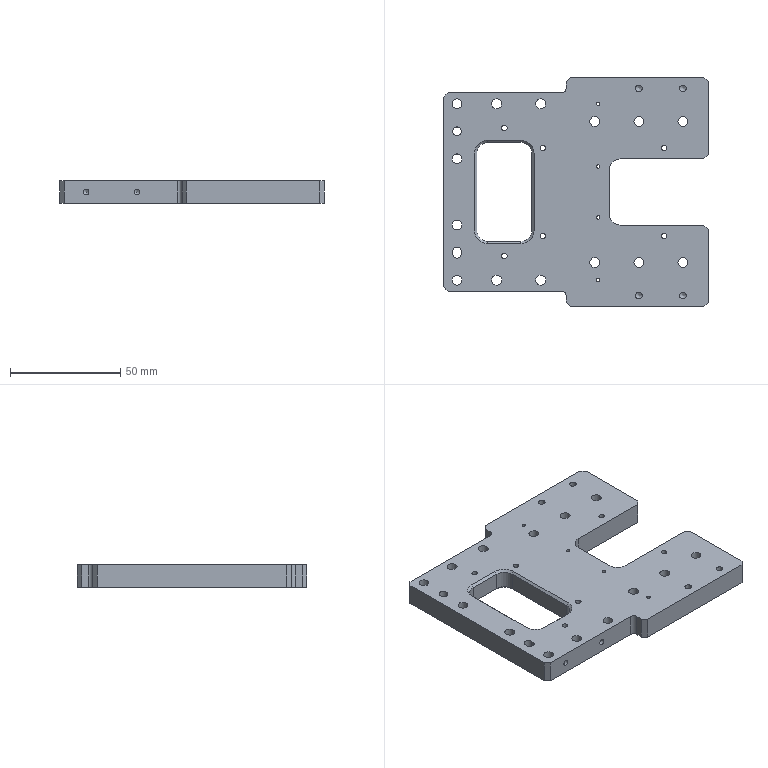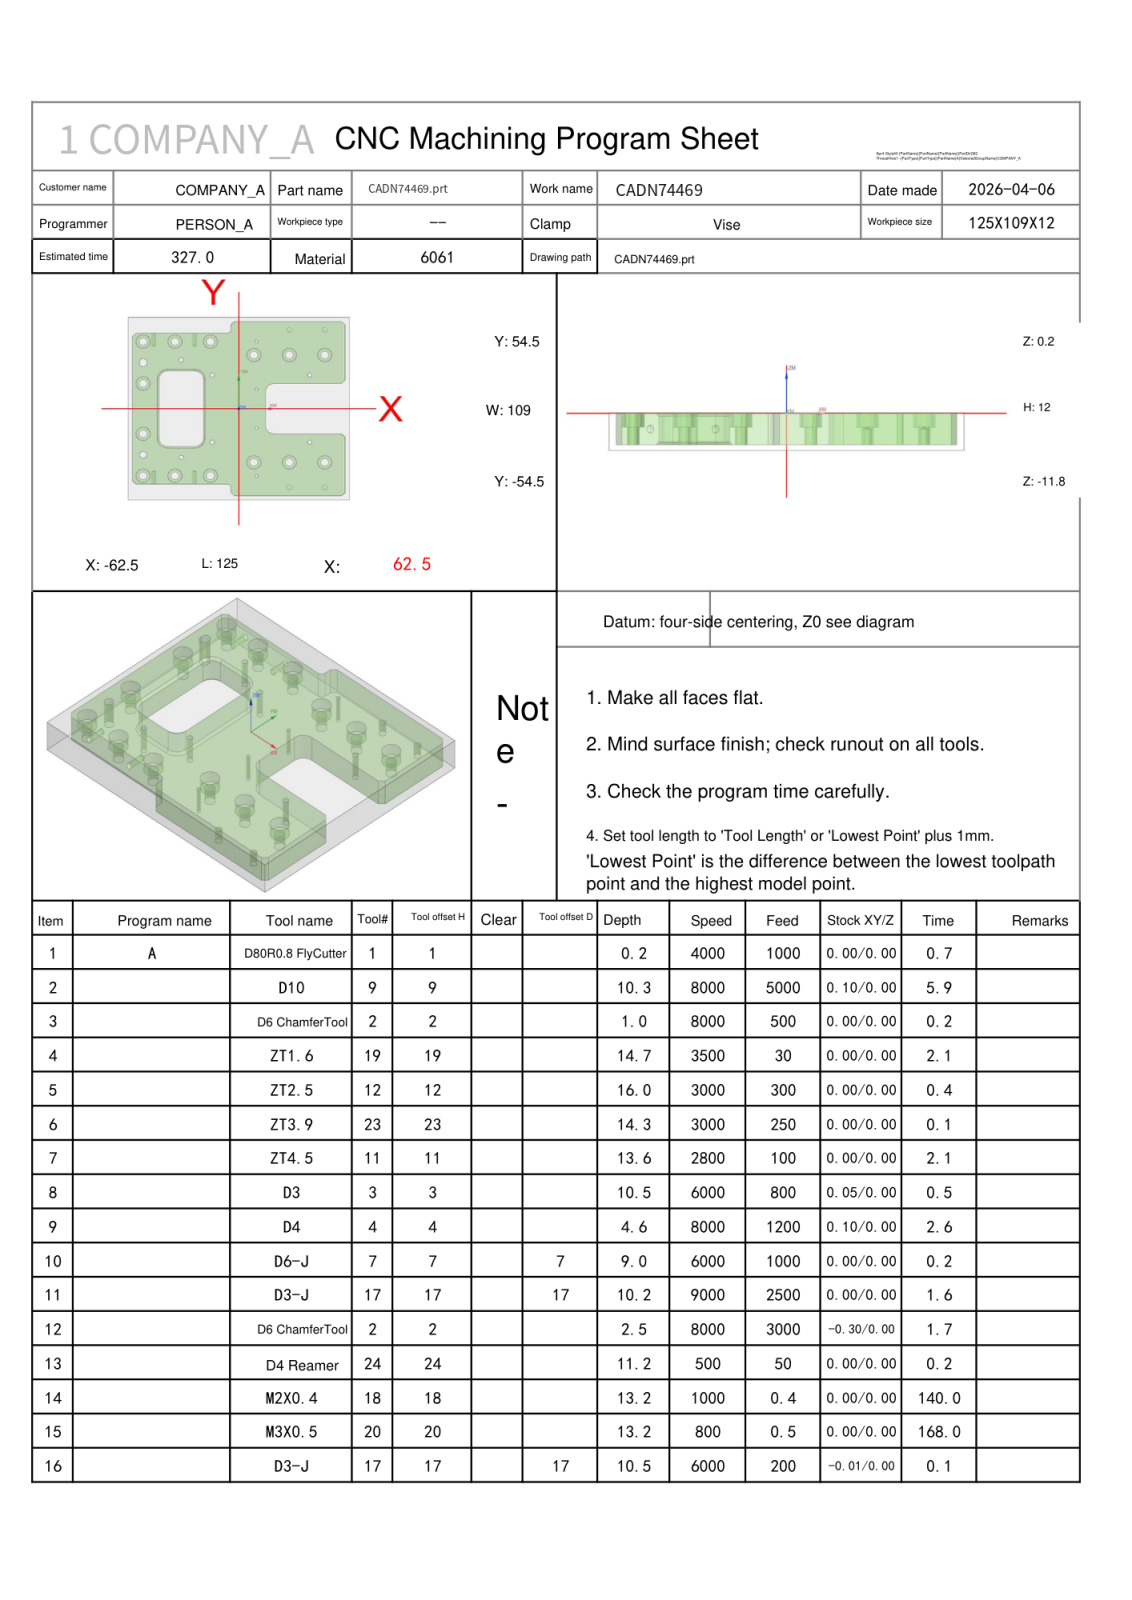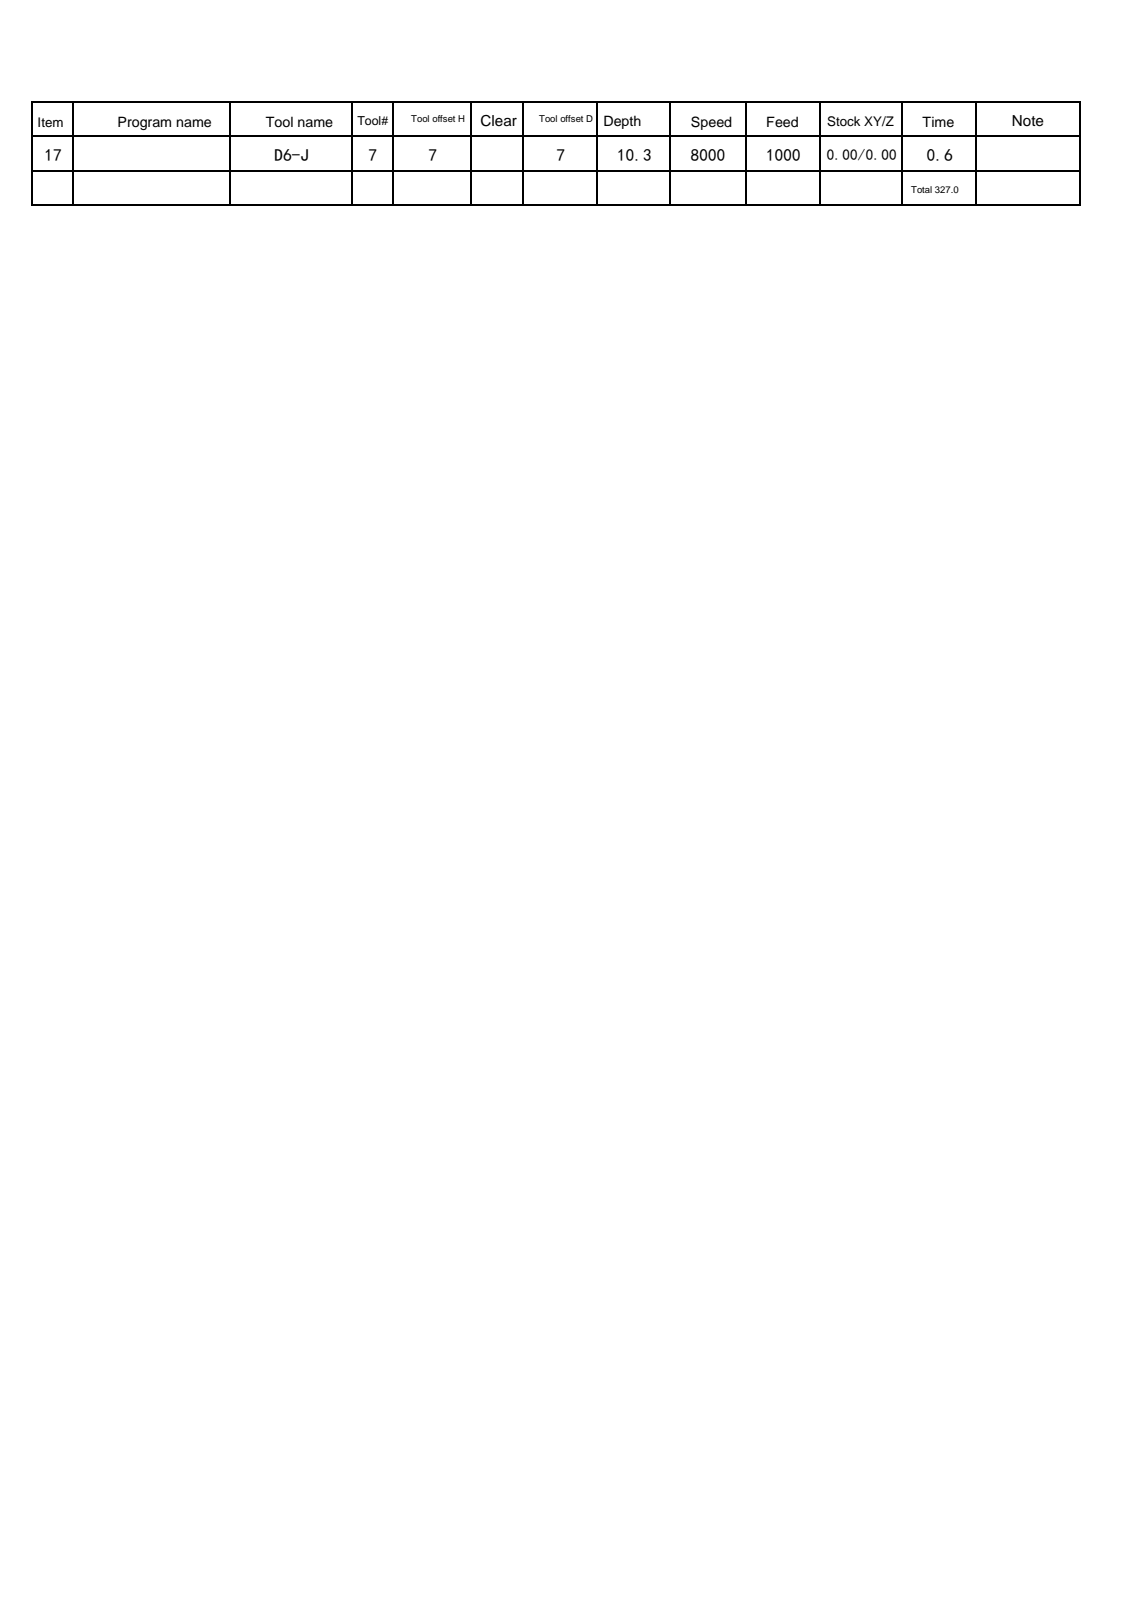NC program | NX | posted by the shop | part box 120 x 104 x 10 mm
Lines 45 to 1202 of 6435:
N2 T09 M06
(D10  D=10. R=0. H=09 ce=0.10 di=0.10)
G00 G90 G54 X74.5 Y7. M03 S8000
G43 H09 Z10.2
M08
Z.719
G01 Z-.481 F5000.
X70.
G03 X63. Y0.0 I0.0 J-7.
G01 Y-10.808
X64.599 Y-12.406
G02 X66.5 Y-17. I-4.599 J-4.594
G01 Y-50.
G02 X64.596 Y-54.596 I-6.5 J0.0
G01 X62.596 Y-56.596
G02 X58. Y-58.5 I-4.596 J4.596
G01 X57.97
X-2.5
G02 X-7.096 Y-56.596 I0.0 J6.5
G01 X-8.692 Y-55.
X-62.5
G02 X-63. Y-54.5 I0.0 J.5
G01 Y-49.192
X-64.596 Y-47.596
G02 X-66.5 Y-43. I4.596 J4.596
G01 Y43.
G02 X-64.596 Y47.596 I6.5 J0.0
G01 X-63. Y49.192
Y54.5
G02 X-62.5 Y55. I.5 J0.0
G01 X-8.692
X-7.096 Y56.596
G02 X-2.5 Y58.5 I4.596 J-4.596
G01 X11.483
X58.002
G02 X62.667 Y56.525 I-.001 J-6.501
G01 X64.596 Y54.596
G02 X66.5 Y50. I-4.596 J-4.596
G01 Y17.
G02 X64.591 Y12.399 I-6.5 J0.0
G01 X63. Y10.808
Y-1.986
G02 X62.582 Y-2.799 I-1. J0.0
G01 X56.333 Y-7.265
G03 X55.957 Y-7.789 I.582 J-.813
G02 X55.003 Y-8.5 I-.957 J.289
G01 X22.497
G02 X21.5 Y-7.503 I.003 J1.
G01 Y7.503
G02 X22.497 Y8.5 I1. J-.003
G01 X54.51
G03 X55.214 Y8.945 I0.0 J.779
G01 X55.382 Y9.3
X55.423 Y9.48
G03 X55.003 Y9.9 I-.42 J0.0
G01 X20.1
Y-9.9
X58.
G02 X61.606 Y-11.394 I0.0 J-5.1
G01 X63.608 Y-13.396
G02 X65.1 Y-17. I-3.608 J-3.604
G01 Y-50.
G02 X63.606 Y-53.606 I-5.1 J0.0
G01 X61.606 Y-55.606
G02 X58. Y-57.1 I-3.606 J3.606
G01 X57.972
X-2.5
G02 X-6.106 Y-55.606 I0.0 J5.1
G01 X-8.106 Y-53.606
G02 X-9.599 Y-50.1 I3.606 J3.606
G01 X-58.
G02 X-61.606 Y-48.606 I0.0 J5.1
G01 X-63.606 Y-46.606
G02 X-65.1 Y-43. I3.606 J3.606
G01 Y43.
G02 X-63.606 Y46.606 I5.1 J0.0
G01 X-61.606 Y48.606
G02 X-59.707 Y49.806 I3.606 J-3.606
X-58.232 Y50.095 I1.691 J-4.72
X-58. Y50.1 I.232 J-5.095
G01 X-9.599
G02 X-8.106 Y53.606 I5.099 J-.1
G01 X-6.106 Y55.606
G02 X-2.5 Y57.1 I3.606 J-3.606
G01 X58.
G02 X61.677 Y55.535 I0.0 J-5.101
G01 X63.606 Y53.606
G02 X65.1 Y50. I-3.606 J-3.606
G01 Y17.
G02 X63.601 Y13.389 I-5.1 J0.0
G01 X61.606 Y11.394
G02 X58.271 Y9.907 I-3.606 J3.606
X57.999 Y9.9 I-.272 J5.094
G01 X57.972
X55.003
G03 X54.583 Y9.48 I0.0 J-.42
G01 X54.623 Y9.3
X54.907 Y8.702
G03 X55.191 Y8.482 I.361 J.172
G02 X56. Y7.503 I-.191 J-.982
G01 Y-1.611
G02 X55.2 Y-2.411 I-.8 J0.0
G01 X55.116 Y-2.406
X46.611 Y-1.506
X46.506 Y-1.5
X29.497
G02 X28.5 Y-.503 I.003 J1.
G01 Y.503
G02 X29.497 Y1.5 I1. J-.003
G01 X48.003
G02 X49. Y.503 I-.003 J-1.
G01 Y-.503
G02 X48.872 Y-.99 I-1. J.003
X48.53 Y-1.348 I-.872 J.49
G03 X46.884 Y-4.316 I1.854 J-2.968
X47.416 Y-6.171 I3.5 J0.0
G01 X74.5
Z.719
G00 Z3.
G01 Y7. F6000.
G00 Z.238
G01 Z-.962 F5000.
X70.
G03 X63. Y0.0 I0.0 J-7.
G01 Y-10.808
X64.599 Y-12.406
G02 X66.5 Y-17. I-4.599 J-4.594
G01 Y-50.
G02 X64.596 Y-54.596 I-6.5 J0.0
G01 X62.596 Y-56.596
G02 X58. Y-58.5 I-4.596 J4.596
G01 X57.972
X-2.5
G02 X-7.096 Y-56.596 I0.0 J6.5
G01 X-8.692 Y-55.
X-62.5
G02 X-63. Y-54.5 I0.0 J.5
G01 Y-49.192
X-64.596 Y-47.596
G02 X-66.5 Y-43. I4.596 J4.596
G01 Y43.
G02 X-64.596 Y47.596 I6.5 J0.0
G01 X-63. Y49.192
Y54.5
G02 X-62.5 Y55. I.5 J0.0
G01 X-8.692
X-7.096 Y56.596
G02 X-2.5 Y58.5 I4.596 J-4.596
G01 X11.483
X58.002
G02 X62.596 Y56.596 I-.002 J-6.5
G01 X64.596 Y54.596
G02 X66.5 Y50. I-4.596 J-4.596
G01 Y17.
G02 X64.596 Y12.404 I-6.5 J0.0
G01 X63. Y10.808
Y-5.
G02 X62.238 Y-5.971 I-1. J0.0
G01 X56.58 Y-7.361
G03 X55.91 Y-7.916 I.239 J-.971
G02 X55.003 Y-8.5 I-.91 J.415
G01 X22.497
G02 X21.5 Y-7.503 I.003 J1.
G01 Y7.503
G02 X22.497 Y8.5 I1. J-.003
G01 X54.511
G03 X55.214 Y8.945 I0.0 J.779
G01 X55.382 Y9.3
X55.423 Y9.48
G03 X55.003 Y9.9 I-.42 J0.0
G01 X20.1
Y-9.9
X58.
G02 X61.606 Y-11.394 I0.0 J-5.1
G01 X63.608 Y-13.396
G02 X65.1 Y-17. I-3.608 J-3.604
G01 Y-50.
G02 X63.606 Y-53.606 I-5.1 J0.0
G01 X61.606 Y-55.606
G02 X58. Y-57.1 I-3.606 J3.606
G01 X57.972
X-2.5
G02 X-6.106 Y-55.606 I0.0 J5.1
G01 X-8.106 Y-53.606
G02 X-9.599 Y-50.1 I3.606 J3.606
G01 X-58.
G02 X-61.606 Y-48.606 I0.0 J5.1
G01 X-63.606 Y-46.606
G02 X-65.1 Y-43. I3.606 J3.606
G01 Y43.
G02 X-63.606 Y46.606 I5.1 J0.0
G01 X-61.606 Y48.606
G02 X-59.707 Y49.806 I3.606 J-3.606
X-58.232 Y50.095 I1.691 J-4.72
X-58. Y50.1 I.232 J-5.095
G01 X-9.599
G02 X-8.106 Y53.606 I5.099 J-.1
G01 X-6.106 Y55.606
G02 X-2.5 Y57.1 I3.606 J-3.606
G01 X58.
G02 X61.606 Y55.606 I0.0 J-5.1
G01 X63.606 Y53.606
G02 X65.1 Y50. I-3.606 J-3.606
G01 Y17.
G02 X63.606 Y13.394 I-5.1 J0.0
G01 X61.606 Y11.394
G02 X58.271 Y9.907 I-3.606 J3.606
G01 X57.972 Y9.9
X55.003
G03 X54.583 Y9.48 I0.0 J-.42
G01 X54.624 Y9.3
X54.907 Y8.702
G03 X55.191 Y8.482 I.361 J.172
G02 X56. Y7.503 I-.191 J-.982
G01 Y-1.611
G02 X55.2 Y-2.411 I-.8 J0.0
G01 X55.116 Y-2.406
X46.611 Y-1.506
X46.506 Y-1.5
X29.497
G02 X28.5 Y-.503 I.003 J1.
G01 Y.503
G02 X29.497 Y1.5 I1. J-.003
G01 X48.003
G02 X49. Y.503 I-.003 J-1.
G01 Y-.503
G02 X48.872 Y-.99 I-1. J.003
X48.53 Y-1.348 I-.872 J.49
G03 X46.884 Y-4.316 I1.854 J-2.968
X47.416 Y-6.171 I3.5 J0.0
G01 X74.5
Z.238
G00 Z2.519
G01 Y7. F6000.
G00 Z-.243
G01 Z-1.443 F5000.
X70.
G03 X63. Y0.0 I0.0 J-7.
G01 Y-10.808
X64.598 Y-12.406
G02 X66.5 Y-17. I-4.598 J-4.594
G01 Y-50.
G02 X64.596 Y-54.596 I-6.5 J0.0
G01 X62.596 Y-56.596
G02 X58. Y-58.5 I-4.596 J4.596
G01 X-2.5
G02 X-7.096 Y-56.596 I0.0 J6.5
G01 X-8.692 Y-55.
X-62.5
G02 X-63. Y-54.5 I0.0 J.5
G01 Y-49.192
X-64.596 Y-47.596
G02 X-66.5 Y-43. I4.596 J4.596
G01 Y43.
G02 X-64.596 Y47.596 I6.5 J0.0
G01 X-63. Y49.192
Y54.5
G02 X-62.5 Y55. I.5 J0.0
G01 X-8.692
X-7.096 Y56.596
G02 X-2.5 Y58.5 I4.596 J-4.596
G01 X58.
G02 X62.596 Y56.596 I0.0 J-6.5
G01 X64.596 Y54.596
G02 X66.5 Y50. I-4.596 J-4.596
G01 Y17.
G02 X64.596 Y12.404 I-6.5 J0.0
G01 X63. Y10.808
Y-5.
G02 X62.238 Y-5.971 I-1. J0.0
G01 X56.58 Y-7.361
G03 X55.91 Y-7.916 I.239 J-.971
G02 X55.003 Y-8.5 I-.91 J.416
G01 X22.497
G02 X21.5 Y-7.503 I.003 J1.
G01 Y7.503
G02 X22.497 Y8.5 I1. J-.003
G01 X54.511
G03 X55.214 Y8.945 I0.0 J.779
G01 X55.383 Y9.3
X55.423 Y9.48
G03 X55.003 Y9.9 I-.42 J0.0
G01 X20.1
Y-9.9
X58.
G02 X61.606 Y-11.394 I0.0 J-5.1
G01 X63.608 Y-13.395
G02 X65.1 Y-17. I-3.608 J-3.605
G01 Y-50.
G02 X63.606 Y-53.606 I-5.1 J0.0
G01 X61.606 Y-55.606
G02 X58. Y-57.1 I-3.606 J3.606
G01 X-2.5
G02 X-6.106 Y-55.606 I0.0 J5.1
G01 X-8.106 Y-53.606
G02 X-9.599 Y-50.1 I3.606 J3.606
G01 X-58.
G02 X-61.606 Y-48.606 I0.0 J5.1
G01 X-63.606 Y-46.606
G02 X-65.1 Y-43. I3.606 J3.606
G01 Y43.
G02 X-63.606 Y46.606 I5.1 J0.0
G01 X-61.606 Y48.606
G02 X-59.707 Y49.806 I3.606 J-3.606
X-58.232 Y50.095 I1.691 J-4.72
X-58. Y50.1 I.232 J-5.095
G01 X-9.599
G02 X-8.106 Y53.606 I5.099 J-.1
G01 X-6.106 Y55.606
G02 X-2.5 Y57.1 I3.606 J-3.606
G01 X58.
G02 X61.606 Y55.606 I0.0 J-5.1
G01 X63.606 Y53.606
G02 X65.1 Y50. I-3.606 J-3.606
G01 Y17.
G02 X63.606 Y13.394 I-5.1 J0.0
G01 X61.606 Y11.394
G02 X58. Y9.9 I-3.606 J3.606
G01 X55.003
G03 X54.583 Y9.48 I0.0 J-.42
G01 X54.624 Y9.3
X54.907 Y8.702
G03 X55.192 Y8.481 I.361 J.172
G02 X56. Y7.503 I-.192 J-.981
G01 Y-1.611
G02 X55.2 Y-2.411 I-.8 J0.0
G01 X55.116 Y-2.406
X46.611 Y-1.506
X46.506 Y-1.5
X29.497
G02 X28.5 Y-.503 I.003 J1.
G01 Y.503
G02 X29.497 Y1.5 I1. J-.003
G01 X48.003
G02 X49. Y.503 I-.003 J-1.
G01 Y-.503
G02 X48.872 Y-.99 I-1. J.003
X48.53 Y-1.348 I-.872 J.49
G03 X46.884 Y-4.316 I1.854 J-2.968
X47.416 Y-6.171 I3.5 J0.0
G01 X74.5
Z-.243
G00 Z2.038
G01 Y7. F6000.
G00 Z-.724
G01 Z-1.924 F5000.
X70.
G03 X63. Y0.0 I0.0 J-7.
G01 Y-10.808
X64.598 Y-12.406
G02 X66.5 Y-17. I-4.598 J-4.594
G01 Y-50.
G02 X64.596 Y-54.596 I-6.5 J0.0
G01 X62.596 Y-56.596
G02 X58. Y-58.5 I-4.596 J4.596
G01 X-2.5
G02 X-7.096 Y-56.596 I0.0 J6.5
G01 X-8.692 Y-55.
X-62.5
G02 X-63. Y-54.5 I0.0 J.5
G01 Y-49.192
X-64.596 Y-47.596
G02 X-66.5 Y-43. I4.596 J4.596
G01 Y43.
G02 X-64.596 Y47.596 I6.5 J0.0
G01 X-63. Y49.192
Y54.5
G02 X-62.5 Y55. I.5 J0.0
G01 X-8.692
X-7.096 Y56.596
G02 X-2.5 Y58.5 I4.596 J-4.596
G01 X58.
G02 X62.596 Y56.596 I0.0 J-6.5
G01 X64.596 Y54.596
G02 X66.5 Y50. I-4.596 J-4.596
G01 Y17.
G02 X64.596 Y12.404 I-6.5 J0.0
G01 X63. Y10.808
Y-5.
G02 X62.239 Y-5.971 I-1. J0.0
G01 X56.58 Y-7.361
G03 X55.91 Y-7.916 I.239 J-.971
G02 X55.003 Y-8.5 I-.91 J.416
G01 X22.497
G02 X21.5 Y-7.503 I.003 J1.
G01 Y7.503
G02 X22.497 Y8.5 I1. J-.003
G01 X54.511
G03 X55.214 Y8.945 I0.0 J.779
G01 X55.383 Y9.3
X55.423 Y9.48
G03 X55.003 Y9.9 I-.42 J0.0
G01 X20.1
Y-9.9
X58.
G02 X61.606 Y-11.394 I0.0 J-5.1
G01 X63.608 Y-13.395
G02 X65.1 Y-17. I-3.608 J-3.605
G01 Y-50.
G02 X63.606 Y-53.606 I-5.1 J0.0
G01 X61.606 Y-55.606
G02 X58. Y-57.1 I-3.606 J3.606
G01 X-2.5
G02 X-6.106 Y-55.606 I0.0 J5.1
G01 X-8.106 Y-53.606
G02 X-9.599 Y-50.1 I3.606 J3.606
G01 X-58.
G02 X-61.606 Y-48.606 I0.0 J5.1
G01 X-63.606 Y-46.606
G02 X-65.1 Y-43. I3.606 J3.606
G01 Y43.
G02 X-63.606 Y46.606 I5.1 J0.0
G01 X-61.606 Y48.606
G02 X-59.707 Y49.806 I3.606 J-3.606
X-58.232 Y50.095 I1.691 J-4.72
X-58. Y50.1 I.232 J-5.095
G01 X-9.599
G02 X-8.106 Y53.606 I5.099 J-.1
G01 X-6.106 Y55.606
G02 X-2.5 Y57.1 I3.606 J-3.606
G01 X58.
G02 X61.606 Y55.606 I0.0 J-5.1
G01 X63.606 Y53.606
G02 X65.1 Y50. I-3.606 J-3.606
G01 Y17.
G02 X63.606 Y13.394 I-5.1 J0.0
G01 X61.606 Y11.394
G02 X58. Y9.9 I-3.606 J3.606
G01 X55.003
G03 X54.583 Y9.48 I0.0 J-.42
G01 X54.624 Y9.3
X54.907 Y8.702
G03 X55.192 Y8.481 I.361 J.172
G02 X56. Y7.503 I-.192 J-.981
G01 Y-1.611
G02 X55.2 Y-2.411 I-.8 J0.0
G01 X55.116 Y-2.406
X46.611 Y-1.506
X46.506 Y-1.5
X29.496
G02 X28.5 Y-.504 I.004 J1.
G01 Y.504
G02 X29.496 Y1.5 I1. J-.004
G01 X48.004
G02 X49. Y.504 I-.004 J-1.
G01 Y-.504
G02 X48.872 Y-.99 I-1. J.004
X48.53 Y-1.348 I-.872 J.49
G03 X46.884 Y-4.316 I1.854 J-2.968
X47.416 Y-6.171 I3.5 J0.0
G01 X74.5
Z-.724
G00 Z1.557
G01 Y7. F6000.
G00 Z-1.205
G01 Z-2.405 F5000.
X70.
G03 X63. Y0.0 I0.0 J-7.
G01 Y-10.808
X64.598 Y-12.406
G02 X66.5 Y-17. I-4.598 J-4.594
G01 Y-50.
G02 X64.596 Y-54.596 I-6.5 J0.0
G01 X62.596 Y-56.596
G02 X58. Y-58.5 I-4.596 J4.596
G01 X-2.5
G02 X-7.096 Y-56.596 I0.0 J6.5
G01 X-8.692 Y-55.
X-62.5
G02 X-63. Y-54.5 I0.0 J.5
G01 Y-49.192
X-64.596 Y-47.596
G02 X-66.5 Y-43. I4.596 J4.596
G01 Y43.
G02 X-64.596 Y47.596 I6.5 J0.0
G01 X-63. Y49.192
Y54.5
G02 X-62.5 Y55. I.5 J0.0
G01 X-8.692
X-7.096 Y56.596
G02 X-2.5 Y58.5 I4.596 J-4.596
G01 X58.
G02 X62.596 Y56.596 I0.0 J-6.5
G01 X64.596 Y54.596
G02 X66.5 Y50. I-4.596 J-4.596
G01 Y17.
G02 X64.596 Y12.404 I-6.5 J0.0
G01 X63. Y10.808
Y-5.
G02 X62.239 Y-5.971 I-1. J0.0
G01 X56.58 Y-7.361
G03 X55.909 Y-7.916 I.239 J-.971
G02 X55.004 Y-8.5 I-.909 J.416
G01 X22.496
G02 X21.5 Y-7.504 I.004 J1.
G01 Y7.504
G02 X22.496 Y8.5 I1. J-.004
G01 X54.511
G03 X55.215 Y8.945 I0.0 J.779
G01 X55.383 Y9.3
X55.424 Y9.48
G03 X55.004 Y9.9 I-.42 J0.0
G01 X20.1
Y-9.9
X58.
G02 X61.606 Y-11.394 I0.0 J-5.1
G01 X63.608 Y-13.395
G02 X65.1 Y-17. I-3.608 J-3.605
G01 Y-50.
G02 X63.606 Y-53.606 I-5.1 J0.0
G01 X61.606 Y-55.606
G02 X58. Y-57.1 I-3.606 J3.606
G01 X-2.5
G02 X-6.106 Y-55.606 I0.0 J5.1
G01 X-8.106 Y-53.606
G02 X-9.599 Y-50.1 I3.606 J3.606
G01 X-58.
G02 X-61.606 Y-48.606 I0.0 J5.1
G01 X-63.606 Y-46.606
G02 X-65.1 Y-43. I3.606 J3.606
G01 Y43.
G02 X-63.606 Y46.606 I5.1 J0.0
G01 X-61.606 Y48.606
G02 X-59.707 Y49.806 I3.606 J-3.606
X-58.232 Y50.095 I1.691 J-4.72
X-58. Y50.1 I.232 J-5.095
G01 X-9.599
G02 X-8.106 Y53.606 I5.099 J-.1
G01 X-6.106 Y55.606
G02 X-2.5 Y57.1 I3.606 J-3.606
G01 X58.
G02 X61.606 Y55.606 I0.0 J-5.1
G01 X63.606 Y53.606
G02 X65.1 Y50. I-3.606 J-3.606
G01 Y17.
G02 X63.606 Y13.394 I-5.1 J0.0
G01 X61.606 Y11.394
G02 X58. Y9.9 I-3.606 J3.606
G01 X55.004
G03 X54.584 Y9.48 I0.0 J-.42
G01 X54.624 Y9.3
X54.908 Y8.702
G03 X55.192 Y8.481 I.361 J.172
G02 X56. Y7.504 I-.192 J-.981
G01 Y-1.611
G02 X55.2 Y-2.411 I-.8 J0.0
G01 X55.116 Y-2.406
X46.611 Y-1.506
X46.506 Y-1.5
X29.496
G02 X28.5 Y-.504 I.004 J1.
G01 Y.504
G02 X29.496 Y1.5 I1. J-.004
G01 X48.004
G02 X49. Y.504 I-.004 J-1.
G01 Y-.504
G02 X48.872 Y-.99 I-1. J.004
X48.53 Y-1.348 I-.872 J.49
G03 X46.884 Y-4.316 I1.854 J-2.968
X47.416 Y-6.171 I3.5 J0.0
G01 X74.5
Z-1.205
G00 Z1.076
G01 Y7. F6000.
G00 Z-1.686
G01 Z-2.886 F5000.
X70.
G03 X63. Y0.0 I0.0 J-7.
G01 Y-10.808
X64.596 Y-12.404
G02 X66.5 Y-17. I-4.596 J-4.596
G01 Y-50.
G02 X64.596 Y-54.596 I-6.5 J0.0
G01 X62.596 Y-56.596
G02 X58. Y-58.5 I-4.596 J4.596
G01 X-2.5
G02 X-7.096 Y-56.596 I0.0 J6.5
G01 X-8.692 Y-55.
X-62.5
G02 X-63. Y-54.5 I0.0 J.5
G01 Y-49.192
X-64.596 Y-47.596
G02 X-66.5 Y-43. I4.596 J4.596
G01 Y43.
G02 X-64.596 Y47.596 I6.5 J0.0
G01 X-63. Y49.192
Y54.5
G02 X-62.5 Y55. I.5 J0.0
G01 X-8.692
X-7.096 Y56.596
G02 X-2.5 Y58.5 I4.596 J-4.596
G01 X58.
G02 X62.596 Y56.596 I0.0 J-6.5
G01 X64.596 Y54.596
G02 X66.5 Y50. I-4.596 J-4.596
G01 Y17.
G02 X64.596 Y12.404 I-6.5 J0.0
G01 X63. Y10.808
Y-5.
G02 X62.239 Y-5.971 I-1. J0.0
G01 X56.58 Y-7.361
G03 X55.909 Y-7.916 I.239 J-.971
G02 X55.004 Y-8.5 I-.909 J.416
G01 X22.496
G02 X21.5 Y-7.504 I.004 J1.
G01 Y7.504
G02 X22.496 Y8.5 I1. J-.004
G01 X54.511
G03 X55.215 Y8.945 I0.0 J.779
G01 X55.383 Y9.3
X55.424 Y9.48
G03 X55.004 Y9.9 I-.42 J0.0
G01 X20.1
Y-9.9
X58.
G02 X61.606 Y-11.394 I0.0 J-5.1
G01 X63.606 Y-13.394
G02 X65.1 Y-17. I-3.606 J-3.606
G01 Y-50.
G02 X63.606 Y-53.606 I-5.1 J0.0
G01 X61.606 Y-55.606
G02 X58. Y-57.1 I-3.606 J3.606
G01 X-2.5
G02 X-6.106 Y-55.606 I0.0 J5.1
G01 X-8.106 Y-53.606
G02 X-9.599 Y-50.1 I3.606 J3.606
G01 X-58.
G02 X-61.606 Y-48.606 I0.0 J5.1
G01 X-63.606 Y-46.606
G02 X-65.1 Y-43. I3.606 J3.606
G01 Y43.
G02 X-63.606 Y46.606 I5.1 J0.0
G01 X-61.606 Y48.606
G02 X-59.707 Y49.806 I3.606 J-3.606
X-58.232 Y50.095 I1.691 J-4.72
X-58. Y50.1 I.232 J-5.095
G01 X-9.599
G02 X-8.106 Y53.606 I5.099 J-.1
G01 X-6.106 Y55.606
G02 X-2.5 Y57.1 I3.606 J-3.606
G01 X58.
G02 X61.606 Y55.606 I0.0 J-5.1
G01 X63.606 Y53.606
G02 X65.1 Y50. I-3.606 J-3.606
G01 Y17.
G02 X63.606 Y13.394 I-5.1 J0.0
G01 X61.606 Y11.394
G02 X58. Y9.9 I-3.606 J3.606
G01 X55.004
G03 X54.584 Y9.48 I0.0 J-.42
G01 X54.624 Y9.3
X54.908 Y8.702
G03 X55.192 Y8.481 I.361 J.172
G02 X56. Y7.504 I-.192 J-.981
G01 Y-1.611
G02 X55.2 Y-2.411 I-.8 J0.0
G01 X55.116 Y-2.406
X46.611 Y-1.506
X46.506 Y-1.5
X29.496
G02 X28.5 Y-.504 I.004 J1.
G01 Y.504
G02 X29.496 Y1.5 I1. J-.004
G01 X48.004
G02 X49. Y.504 I-.004 J-1.
G01 Y-.504
G02 X48.872 Y-.99 I-1. J.004
X48.53 Y-1.348 I-.872 J.49
G03 X46.884 Y-4.316 I1.854 J-2.968
X47.416 Y-6.171 I3.5 J0.0
G01 X74.5
Z-1.686
G00 Z.595
G01 Y7. F6000.
G00 Z-2.167
G01 Z-3.367 F5000.
X70.
G03 X63. Y0.0 I0.0 J-7.
G01 Y-10.808
X64.596 Y-12.404
G02 X66.5 Y-17. I-4.596 J-4.596
G01 Y-50.
G02 X64.596 Y-54.596 I-6.5 J0.0
G01 X62.596 Y-56.596
G02 X58. Y-58.5 I-4.596 J4.596
G01 X-2.5
G02 X-7.096 Y-56.596 I0.0 J6.5
G01 X-8.692 Y-55.
X-62.5
G02 X-63. Y-54.5 I0.0 J.5
G01 Y-49.192
X-64.596 Y-47.596
G02 X-66.5 Y-43. I4.596 J4.596
G01 Y43.
G02 X-64.596 Y47.596 I6.5 J0.0
G01 X-63. Y49.192
Y54.5
G02 X-62.5 Y55. I.5 J0.0
G01 X-8.692
X-7.096 Y56.596
G02 X-2.5 Y58.5 I4.596 J-4.596
G01 X58.
G02 X62.596 Y56.596 I0.0 J-6.5
G01 X64.596 Y54.596
G02 X66.5 Y50. I-4.596 J-4.596
G01 Y17.
G02 X64.596 Y12.404 I-6.5 J0.0
G01 X63. Y10.808
Y-5.
G02 X62.239 Y-5.971 I-1. J0.0
G01 X56.579 Y-7.362
G03 X55.909 Y-7.916 I.239 J-.971
G02 X55.004 Y-8.5 I-.909 J.416
G01 X22.496
G02 X21.5 Y-7.504 I.004 J1.
G01 Y7.504
G02 X22.496 Y8.5 I1. J-.004
G01 X54.512
G03 X55.215 Y8.945 I0.0 J.779
G01 X55.383 Y9.3
X55.424 Y9.48
G03 X55.004 Y9.9 I-.42 J0.0
G01 X20.1
Y-9.9
X58.
G02 X61.606 Y-11.394 I0.0 J-5.1
G01 X63.606 Y-13.394
G02 X65.1 Y-17. I-3.606 J-3.606
G01 Y-50.
G02 X63.606 Y-53.606 I-5.1 J0.0
G01 X61.606 Y-55.606
G02 X58. Y-57.1 I-3.606 J3.606
G01 X-2.5
G02 X-6.106 Y-55.606 I0.0 J5.1
G01 X-8.106 Y-53.606
G02 X-9.599 Y-50.1 I3.606 J3.606
G01 X-58.
G02 X-61.606 Y-48.606 I0.0 J5.1
G01 X-63.606 Y-46.606
G02 X-65.1 Y-43. I3.606 J3.606
G01 Y43.
G02 X-63.606 Y46.606 I5.1 J0.0
G01 X-61.606 Y48.606
G02 X-59.707 Y49.806 I3.606 J-3.606
X-58.232 Y50.095 I1.691 J-4.72
X-58. Y50.1 I.232 J-5.095
G01 X-9.599
G02 X-8.106 Y53.606 I5.099 J-.1
G01 X-6.106 Y55.606
G02 X-2.5 Y57.1 I3.606 J-3.606
G01 X58.
G02 X61.606 Y55.606 I0.0 J-5.1
G01 X63.606 Y53.606
G02 X65.1 Y50. I-3.606 J-3.606
G01 Y17.
G02 X63.606 Y13.394 I-5.1 J0.0
G01 X61.606 Y11.394
G02 X58. Y9.9 I-3.606 J3.606
G01 X55.004
G03 X54.584 Y9.48 I0.0 J-.42
G01 X54.624 Y9.3
X54.908 Y8.702
G03 X55.192 Y8.481 I.361 J.172
G02 X56. Y7.504 I-.192 J-.981
G01 Y-1.611
G02 X55.2 Y-2.411 I-.8 J0.0
G01 X55.116 Y-2.406
X46.611 Y-1.506
X46.506 Y-1.5
X29.496
G02 X28.5 Y-.504 I.004 J1.
G01 Y.504
G02 X29.496 Y1.5 I1. J-.004
G01 X48.004
G02 X49. Y.504 I-.004 J-1.
G01 Y-.504
G02 X48.872 Y-.99 I-1. J.004
X48.53 Y-1.348 I-.872 J.49
G03 X46.884 Y-4.316 I1.854 J-2.968
X47.416 Y-6.171 I3.5 J0.0
G01 X74.5
Z-2.167
G00 Z.114
G01 Y7. F6000.
G00 Z-2.648
G01 Z-3.848 F5000.
X70.
G03 X63. Y0.0 I0.0 J-7.
G01 Y-10.808
X64.596 Y-12.404
G02 X66.5 Y-17. I-4.596 J-4.596
G01 Y-50.
G02 X64.596 Y-54.596 I-6.5 J0.0
G01 X62.596 Y-56.596
G02 X58. Y-58.5 I-4.596 J4.596
G01 X-2.5
G02 X-7.096 Y-56.596 I0.0 J6.5
G01 X-8.692 Y-55.
X-62.5
G02 X-63. Y-54.5 I0.0 J.5
G01 Y-49.192
X-64.596 Y-47.596
G02 X-66.5 Y-43. I4.596 J4.596
G01 Y43.
G02 X-64.596 Y47.596 I6.5 J0.0
G01 X-63. Y49.192
Y54.5
G02 X-62.5 Y55. I.5 J0.0
G01 X-8.692
X-7.096 Y56.596
G02 X-2.5 Y58.5 I4.596 J-4.596
G01 X58.
G02 X62.596 Y56.596 I0.0 J-6.5
G01 X64.596 Y54.596
G02 X66.5 Y50. I-4.596 J-4.596
G01 Y17.
G02 X64.596 Y12.404 I-6.5 J0.0
G01 X63. Y10.808
Y-5.
G02 X62.239 Y-5.971 I-1. J0.0
G01 X56.579 Y-7.362
G03 X55.909 Y-7.916 I.239 J-.971
G02 X55.004 Y-8.5 I-.909 J.416
G01 X22.496
G02 X21.5 Y-7.504 I.004 J1.
G01 Y7.504
G02 X22.496 Y8.5 I1. J-.004
G01 X54.512
G03 X55.215 Y8.945 I0.0 J.779
G01 X55.384 Y9.3
X55.424 Y9.48
G03 X55.004 Y9.9 I-.42 J0.0
G01 X20.1
Y-9.9
X58.
G02 X61.606 Y-11.394 I0.0 J-5.1
G01 X63.606 Y-13.394
G02 X65.1 Y-17. I-3.606 J-3.606
G01 Y-50.
G02 X63.606 Y-53.606 I-5.1 J0.0
G01 X61.606 Y-55.606
G02 X58. Y-57.1 I-3.606 J3.606
G01 X-2.5
G02 X-6.106 Y-55.606 I0.0 J5.1
G01 X-8.106 Y-53.606
G02 X-9.599 Y-50.1 I3.606 J3.606
G01 X-58.
G02 X-61.606 Y-48.606 I0.0 J5.1
G01 X-63.606 Y-46.606
G02 X-65.1 Y-43. I3.606 J3.606
G01 Y43.
G02 X-63.606 Y46.606 I5.1 J0.0
G01 X-61.606 Y48.606
G02 X-59.707 Y49.806 I3.606 J-3.606
X-58.232 Y50.095 I1.69 J-4.72
X-58. Y50.1 I.232 J-5.095
G01 X-9.599
G02 X-8.106 Y53.606 I5.099 J-.1
G01 X-6.106 Y55.606
G02 X-2.5 Y57.1 I3.606 J-3.606
G01 X58.
G02 X61.606 Y55.606 I0.0 J-5.1
G01 X63.606 Y53.606
G02 X65.1 Y50. I-3.606 J-3.606
G01 Y17.
G02 X63.606 Y13.394 I-5.1 J0.0
G01 X61.606 Y11.394
G02 X58. Y9.9 I-3.606 J3.606
G01 X55.004
G03 X54.584 Y9.48 I0.0 J-.42
G01 X54.625 Y9.3
X54.908 Y8.702
G03 X55.192 Y8.481 I.361 J.172
G02 X56. Y7.504 I-.192 J-.981
G01 Y-1.611
G02 X55.2 Y-2.411 I-.8 J0.0
G01 X55.116 Y-2.406
X46.611 Y-1.506
X46.506 Y-1.5
X29.496
G02 X28.5 Y-.504 I.004 J1.
G01 Y.504
G02 X29.496 Y1.5 I1. J-.004
G01 X48.004
G02 X49. Y.504 I-.004 J-1.
G01 Y-.504
G02 X48.872 Y-.99 I-1. J.004
X48.53 Y-1.348 I-.872 J.49
G03 X46.884 Y-4.316 I1.854 J-2.968
X47.416 Y-6.171 I3.5 J0.0
G01 X74.5
Z-2.648
G00 Z-.367
G01 Y7. F6000.
G00 Z-3.129
G01 Z-4.329 F5000.
X70.
G03 X63. Y0.0 I0.0 J-7.
G01 Y-10.808
X64.596 Y-12.404
G02 X66.5 Y-17. I-4.596 J-4.596
G01 Y-50.
G02 X64.596 Y-54.596 I-6.5 J0.0
G01 X62.596 Y-56.596
G02 X58. Y-58.5 I-4.596 J4.596
G01 X-2.5
G02 X-7.096 Y-56.596 I0.0 J6.5
G01 X-8.692 Y-55.
X-62.5
G02 X-63. Y-54.5 I0.0 J.5
G01 Y-49.192
X-64.596 Y-47.596
G02 X-66.5 Y-43. I4.596 J4.596
G01 Y43.
G02 X-64.596 Y47.596 I6.5 J0.0
G01 X-63. Y49.192
Y54.5
G02 X-62.5 Y55. I.5 J0.0
G01 X-8.692
X-7.096 Y56.596
G02 X-2.5 Y58.5 I4.596 J-4.596
G01 X58.
G02 X62.596 Y56.596 I0.0 J-6.5
G01 X64.596 Y54.596
G02 X66.5 Y50. I-4.596 J-4.596
G01 Y17.
G02 X64.596 Y12.404 I-6.5 J0.0
G01 X63. Y10.808
Y-5.
G02 X62.239 Y-5.971 I-1. J0.0
G01 X56.579 Y-7.362
G03 X55.909 Y-7.916 I.239 J-.971
G02 X55.004 Y-8.5 I-.909 J.416
G01 X22.496
G02 X21.5 Y-7.504 I.004 J1.
G01 Y7.504
G02 X22.496 Y8.5 I1. J-.004
G01 X54.512
G03 X55.215 Y8.945 I0.0 J.779
G01 X55.384 Y9.3
X55.424 Y9.48
G03 X55.004 Y9.9 I-.42 J0.0
G01 X20.1
Y-9.9
X58.
G02 X61.606 Y-11.394 I0.0 J-5.1
G01 X63.606 Y-13.394
G02 X65.1 Y-17. I-3.606 J-3.606
G01 Y-50.
G02 X63.606 Y-53.606 I-5.1 J0.0
G01 X61.606 Y-55.606
G02 X58. Y-57.1 I-3.606 J3.606
G01 X-2.5
G02 X-6.106 Y-55.606 I0.0 J5.1
G01 X-8.106 Y-53.606
G02 X-9.599 Y-50.1 I3.606 J3.606
G01 X-58.
G02 X-61.606 Y-48.606 I0.0 J5.1
G01 X-63.606 Y-46.606
G02 X-65.1 Y-43. I3.606 J3.606
G01 Y43.
G02 X-63.606 Y46.606 I5.1 J0.0
G01 X-61.606 Y48.606
G02 X-59.707 Y49.806 I3.606 J-3.606
X-58.232 Y50.095 I1.69 J-4.72
X-58. Y50.1 I.232 J-5.095
G01 X-9.599
G02 X-8.106 Y53.606 I5.099 J-.1
G01 X-6.106 Y55.606
G02 X-2.5 Y57.1 I3.606 J-3.606
G01 X58.
G02 X61.606 Y55.606 I0.0 J-5.1
G01 X63.606 Y53.606
G02 X65.1 Y50. I-3.606 J-3.606
G01 Y17.
G02 X63.606 Y13.394 I-5.1 J0.0
G01 X61.606 Y11.394
G02 X58. Y9.9 I-3.606 J3.606
G01 X55.004
G03 X54.584 Y9.48 I0.0 J-.42
G01 X54.625 Y9.3
X54.908 Y8.702
G03 X55.192 Y8.481 I.361 J.172
G02 X56. Y7.504 I-.192 J-.981
G01 Y-1.611
G02 X55.2 Y-2.411 I-.8 J0.0
G01 X55.116 Y-2.406
X46.611 Y-1.506
X46.506 Y-1.5
X29.496
G02 X28.5 Y-.504 I.004 J1.
G01 Y.504
G02 X29.496 Y1.5 I1. J-.004
G01 X48.004
G02 X49. Y.504 I-.004 J-1.
G01 Y-.504
G02 X48.872 Y-.99 I-1. J.004
X48.53 Y-1.348 I-.872 J.49
G03 X46.884 Y-4.316 I1.854 J-2.968
X47.416 Y-6.171 I3.5 J0.0
G01 X74.5
Z-3.129
G00 Z-.848
G01 Y7. F6000.
G00 Z-3.61
G01 Z-4.81 F5000.
X70.
G03 X63. Y0.0 I0.0 J-7.
G01 Y-10.808
X64.596 Y-12.404
G02 X66.5 Y-17. I-4.596 J-4.596
G01 Y-50.
G02 X64.596 Y-54.596 I-6.5 J0.0
G01 X62.596 Y-56.596
G02 X58. Y-58.5 I-4.596 J4.596
G01 X-2.5
G02 X-7.096 Y-56.596 I0.0 J6.5
G01 X-8.692 Y-55.
X-62.5
G02 X-63. Y-54.5 I0.0 J.5
G01 Y-49.192
X-64.596 Y-47.596
G02 X-66.5 Y-43. I4.596 J4.596
G01 Y43.
G02 X-64.596 Y47.596 I6.5 J0.0
G01 X-63. Y49.192
Y54.5
G02 X-62.5 Y55. I.5 J0.0
G01 X-8.692
X-7.096 Y56.596
G02 X-2.5 Y58.5 I4.596 J-4.596
G01 X58.
G02 X62.596 Y56.596 I0.0 J-6.5
G01 X64.596 Y54.596
G02 X66.5 Y50. I-4.596 J-4.596
G01 Y17.
G02 X64.596 Y12.404 I-6.5 J0.0
G01 X63. Y10.808
Y-5.
G02 X62.239 Y-5.971 I-1. J0.0
G01 X56.579 Y-7.362
G03 X55.909 Y-7.916 I.239 J-.971
G02 X55.004 Y-8.5 I-.909 J.416
G01 X22.496
G02 X21.5 Y-7.504 I.004 J1.
G01 Y7.504
G02 X22.496 Y8.5 I1. J-.004
G01 X54.512
G03 X55.215 Y8.945 I0.0 J.779
G01 X55.384 Y9.3
X55.424 Y9.48
G03 X55.004 Y9.9 I-.42 J0.0
G01 X20.1
Y-9.9
X58.
G02 X61.606 Y-11.394 I0.0 J-5.1
G01 X63.606 Y-13.394
G02 X65.1 Y-17. I-3.606 J-3.606
G01 Y-50.
G02 X63.606 Y-53.606 I-5.1 J0.0
G01 X61.606 Y-55.606
G02 X58. Y-57.1 I-3.606 J3.606
G01 X-2.5
G02 X-6.106 Y-55.606 I0.0 J5.1
G01 X-8.106 Y-53.606
G02 X-9.599 Y-50.1 I3.606 J3.606
G01 X-58.
G02 X-61.606 Y-48.606 I0.0 J5.1
G01 X-63.606 Y-46.606
G02 X-65.1 Y-43. I3.606 J3.606
G01 Y43.
G02 X-63.606 Y46.606 I5.1 J0.0
G01 X-61.606 Y48.606
G02 X-59.707 Y49.806 I3.606 J-3.606
X-58.232 Y50.095 I1.69 J-4.72
X-58. Y50.1 I.232 J-5.095
G01 X-9.599
G02 X-8.106 Y53.606 I5.099 J-.1
G01 X-6.106 Y55.606
G02 X-2.5 Y57.1 I3.606 J-3.606
G01 X58.
G02 X61.606 Y55.606 I0.0 J-5.1
G01 X63.606 Y53.606
G02 X65.1 Y50. I-3.606 J-3.606
G01 Y17.
G02 X63.606 Y13.394 I-5.1 J0.0
G01 X61.606 Y11.394
G02 X58. Y9.9 I-3.606 J3.606
G01 X55.004
G03 X54.584 Y9.48 I0.0 J-.42
G01 X54.625 Y9.3
X54.908 Y8.702
G03 X55.193 Y8.481 I.361 J.172
G02 X56. Y7.504 I-.193 J-.981
G01 Y-1.611
G02 X55.2 Y-2.411 I-.8 J0.0
G01 X55.116 Y-2.406
X46.611 Y-1.506
X46.506 Y-1.5
X29.495
G02 X28.5 Y-.505 I.005 J1.
G01 Y.505
G02 X29.495 Y1.5 I1. J-.005
G01 X48.005
G02 X49. Y.505 I-.005 J-1.
G01 Y-.505
G02 X48.872 Y-.99 I-1. J.005
X48.53 Y-1.348 I-.872 J.49
G03 X46.884 Y-4.316 I1.854 J-2.968
X47.416 Y-6.171 I3.5 J0.0
G01 X74.5
Z-3.61
G00 Z-1.329
G01 Y7. F6000.
G00 Z-4.09
G01 Z-5.29 F5000.
X70.
G03 X63. Y0.0 I0.0 J-7.
G01 Y-10.808
X64.596 Y-12.404
G02 X66.5 Y-17. I-4.596 J-4.596
G01 Y-50.
G02 X64.596 Y-54.596 I-6.5 J0.0
G01 X62.596 Y-56.596
G02 X58. Y-58.5 I-4.596 J4.596
G01 X-2.5
G02 X-7.096 Y-56.596 I0.0 J6.5
G01 X-8.692 Y-55.
X-62.5
G02 X-63. Y-54.5 I0.0 J.5
G01 Y-49.192
X-64.596 Y-47.596
G02 X-66.5 Y-43. I4.596 J4.596
G01 Y43.
G02 X-64.596 Y47.596 I6.5 J0.0
G01 X-63. Y49.192
Y54.5
G02 X-62.5 Y55. I.5 J0.0
G01 X-8.692
X-7.096 Y56.596
G02 X-2.5 Y58.5 I4.596 J-4.596
G01 X58.
G02 X62.596 Y56.596 I0.0 J-6.5
G01 X64.596 Y54.596
G02 X66.5 Y50. I-4.596 J-4.596
G01 Y17.
G02 X64.596 Y12.404 I-6.5 J0.0
G01 X63. Y10.808
Y-5.
G02 X62.239 Y-5.971 I-1. J0.0
G01 X56.579 Y-7.362
G03 X55.909 Y-7.916 I.239 J-.971
G02 X55.005 Y-8.5 I-.909 J.416
G01 X22.495
G02 X21.5 Y-7.505 I.004 J1.
G01 Y7.505
G02 X22.495 Y8.5 I1. J-.004
G01 X54.512